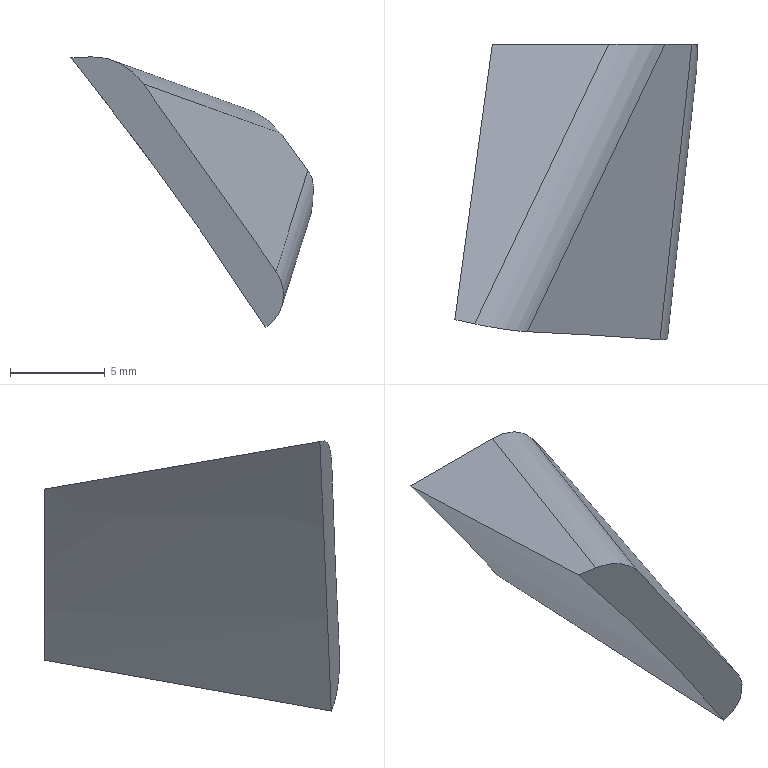Part | STEP file | solid 13 | 1 solid | 10 faces | box 12.797 x 15.596 x 14.273 mm | volume 763.699 mm3 | plane 4 | cylinder 4 | spline 1 | other 1 | commonest cylinder face diameters 4 x1 6 x1 12 x1 15 x1